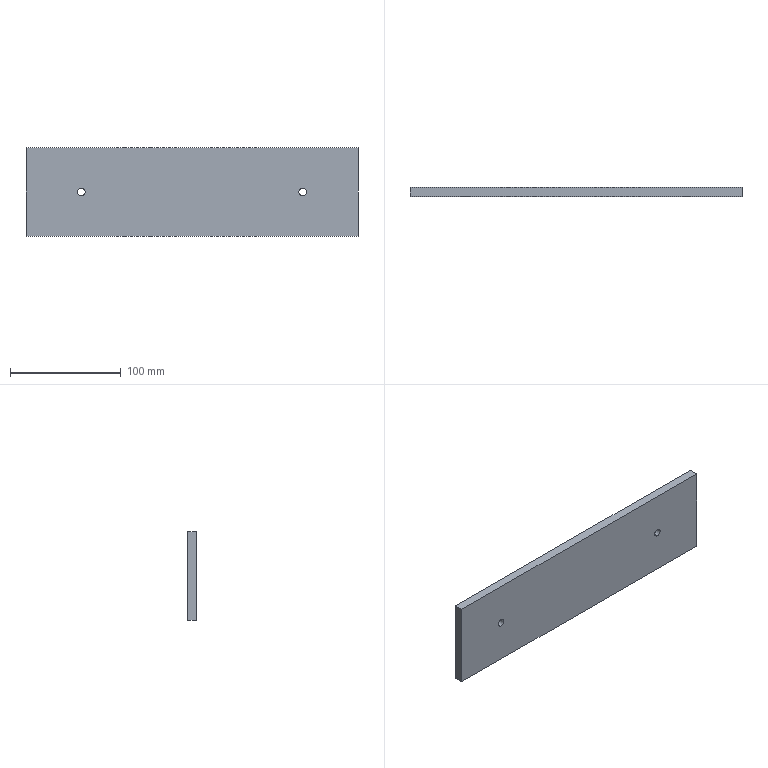Part | SolidWorks | features Extrusion 1, HoleWzd 1 | 1 solid | 10 faces | box 300 x 8 x 80 mm | volume 191419 mm3 | plane 6 | cylinder 4 | commonest cylinder face diameters 6.8 x4
STEP:
#1=CARTESIAN_POINT('',(50.,0.,-43.4));
#2=VERTEX_POINT('',#1);
#3=CARTESIAN_POINT('',(50.,0.,-36.6));
#4=VERTEX_POINT('',#3);
#5=CARTESIAN_POINT('',(50.,0.,-40.));
#6=DIRECTION('',(0.,1.,0.));
#7=DIRECTION('',(0.,0.,1.));
#8=AXIS2_PLACEMENT_3D('',#5,#6,#7);
#9=CIRCLE('',#8,3.4);
#10=EDGE_CURVE('',#2,#4,#9,.T.);
#11=ORIENTED_EDGE('',*,*,#10,.F.);
#12=CARTESIAN_POINT('',(50.,8.,-43.4));
#13=VERTEX_POINT('',#12);
#14=CARTESIAN_POINT('',(50.,8.,-43.4));
#15=DIRECTION('',(0.,1.,0.));
#16=VECTOR('',#15,1000.);
#17=LINE('',#14,#16);
#18=EDGE_CURVE('',#2,#13,#17,.T.);
#19=ORIENTED_EDGE('',*,*,#18,.T.);
#20=CARTESIAN_POINT('',(50.,8.,-36.6));
#21=VERTEX_POINT('',#20);
#22=CARTESIAN_POINT('',(50.,8.,-40.));
#23=DIRECTION('',(0.,1.,0.));
#24=DIRECTION('',(0.,0.,1.));
#25=AXIS2_PLACEMENT_3D('',#22,#23,#24);
#26=CIRCLE('',#25,3.4);
#27=EDGE_CURVE('',#13,#21,#26,.T.);
#28=ORIENTED_EDGE('',*,*,#27,.T.);
#29=CARTESIAN_POINT('',(50.,8.,-36.6));
#30=DIRECTION('',(0.,1.,0.));
#31=VECTOR('',#30,1000.);
#32=LINE('',#29,#31);
#33=EDGE_CURVE('',#4,#21,#32,.T.);
#34=ORIENTED_EDGE('',*,*,#33,.F.);
#35=EDGE_LOOP('',(#11,#19,#28,#34));
#36=FACE_OUTER_BOUND('',#35,.T.);
#37=CARTESIAN_POINT('',(50.,8.,-40.));
#38=DIRECTION('',(0.,1.,0.));
#39=DIRECTION('',(0.,0.,1.));
#40=AXIS2_PLACEMENT_3D('',#37,#38,#39);
#41=CYLINDRICAL_SURFACE('',#40,3.4);
#42=ADVANCED_FACE('',(#36),#41,.F.);
#43=CARTESIAN_POINT('',(250.,0.,-43.4));
#44=VERTEX_POINT('',#43);
#45=CARTESIAN_POINT('',(250.,0.,-36.6));
#46=VERTEX_POINT('',#45);
#47=CARTESIAN_POINT('',(250.,0.,-40.));
#48=DIRECTION('',(0.,1.,0.));
#49=DIRECTION('',(0.,0.,1.));
#50=AXIS2_PLACEMENT_3D('',#47,#48,#49);
#51=CIRCLE('',#50,3.4);
#52=EDGE_CURVE('',#44,#46,#51,.T.);
#53=ORIENTED_EDGE('',*,*,#52,.F.);
#54=CARTESIAN_POINT('',(250.,8.,-43.4));
#55=VERTEX_POINT('',#54);
#56=CARTESIAN_POINT('',(250.,8.,-43.4));
#57=DIRECTION('',(0.,1.,0.));
#58=VECTOR('',#57,1000.);
#59=LINE('',#56,#58);
#60=EDGE_CURVE('',#44,#55,#59,.T.);
#61=ORIENTED_EDGE('',*,*,#60,.T.);
#62=CARTESIAN_POINT('',(250.,8.,-36.6));
#63=VERTEX_POINT('',#62);
#64=CARTESIAN_POINT('',(250.,8.,-40.));
#65=DIRECTION('',(0.,1.,0.));
#66=DIRECTION('',(0.,0.,1.));
#67=AXIS2_PLACEMENT_3D('',#64,#65,#66);
#68=CIRCLE('',#67,3.4);
#69=EDGE_CURVE('',#55,#63,#68,.T.);
#70=ORIENTED_EDGE('',*,*,#69,.T.);
#71=CARTESIAN_POINT('',(250.,8.,-36.6));
#72=DIRECTION('',(0.,1.,0.));
#73=VECTOR('',#72,1000.);
#74=LINE('',#71,#73);
#75=EDGE_CURVE('',#46,#63,#74,.T.);
#76=ORIENTED_EDGE('',*,*,#75,.F.);
#77=EDGE_LOOP('',(#53,#61,#70,#76));
#78=FACE_OUTER_BOUND('',#77,.T.);
#79=CARTESIAN_POINT('',(250.,8.,-40.));
#80=DIRECTION('',(0.,1.,0.));
#81=DIRECTION('',(0.,0.,1.));
#82=AXIS2_PLACEMENT_3D('',#79,#80,#81);
#83=CYLINDRICAL_SURFACE('',#82,3.4);
#84=ADVANCED_FACE('',(#78),#83,.F.);
#85=CARTESIAN_POINT('',(0.,0.,-80.));
#86=VERTEX_POINT('',#85);
#87=CARTESIAN_POINT('',(0.,0.,0.));
#88=VERTEX_POINT('',#87);
#89=CARTESIAN_POINT('',(0.,0.,0.));
#90=DIRECTION('',(0.,0.,1.));
#91=VECTOR('',#90,1000.);
#92=LINE('',#89,#91);
#93=EDGE_CURVE('',#86,#88,#92,.T.);
#94=ORIENTED_EDGE('',*,*,#93,.T.);
#95=CARTESIAN_POINT('',(0.,8.,0.));
#96=VERTEX_POINT('',#95);
#97=CARTESIAN_POINT('',(0.,8.,0.));
#98=DIRECTION('',(0.,-1.,0.));
#99=VECTOR('',#98,1000.);
#100=LINE('',#97,#99);
#101=EDGE_CURVE('',#96,#88,#100,.T.);
#102=ORIENTED_EDGE('',*,*,#101,.F.);
#103=CARTESIAN_POINT('',(0.,8.,-80.));
#104=VERTEX_POINT('',#103);
#105=CARTESIAN_POINT('',(0.,8.,0.));
#106=DIRECTION('',(0.,0.,1.));
#107=VECTOR('',#106,1000.);
#108=LINE('',#105,#107);
#109=EDGE_CURVE('',#104,#96,#108,.T.);
#110=ORIENTED_EDGE('',*,*,#109,.F.);
#111=CARTESIAN_POINT('',(0.,8.,-80.));
#112=DIRECTION('',(0.,-1.,0.));
#113=VECTOR('',#112,1000.);
#114=LINE('',#111,#113);
#115=EDGE_CURVE('',#104,#86,#114,.T.);
#116=ORIENTED_EDGE('',*,*,#115,.T.);
#117=EDGE_LOOP('',(#94,#102,#110,#116));
#118=FACE_OUTER_BOUND('',#117,.T.);
#119=CARTESIAN_POINT('',(0.,8.,0.));
#120=DIRECTION('',(1.,0.,0.));
#121=DIRECTION('',(0.,0.,-1.));
#122=AXIS2_PLACEMENT_3D('',#119,#120,#121);
#123=PLANE('',#122);
#124=ADVANCED_FACE('',(#118),#123,.F.);
#125=CARTESIAN_POINT('',(300.,0.,0.));
#126=VERTEX_POINT('',#125);
#127=CARTESIAN_POINT('',(0.,0.,0.));
#128=DIRECTION('',(1.,0.,0.));
#129=VECTOR('',#128,1000.);
#130=LINE('',#127,#129);
#131=EDGE_CURVE('',#88,#126,#130,.T.);
#132=ORIENTED_EDGE('',*,*,#131,.T.);
#133=CARTESIAN_POINT('',(300.,8.,0.));
#134=VERTEX_POINT('',#133);
#135=CARTESIAN_POINT('',(300.,8.,0.));
#136=DIRECTION('',(0.,-1.,0.));
#137=VECTOR('',#136,1000.);
#138=LINE('',#135,#137);
#139=EDGE_CURVE('',#134,#126,#138,.T.);
#140=ORIENTED_EDGE('',*,*,#139,.F.);
#141=CARTESIAN_POINT('',(0.,8.,0.));
#142=DIRECTION('',(1.,0.,0.));
#143=VECTOR('',#142,1000.);
#144=LINE('',#141,#143);
#145=EDGE_CURVE('',#96,#134,#144,.T.);
#146=ORIENTED_EDGE('',*,*,#145,.F.);
#147=ORIENTED_EDGE('',*,*,#101,.T.);
#148=EDGE_LOOP('',(#132,#140,#146,#147));
#149=FACE_OUTER_BOUND('',#148,.T.);
#150=CARTESIAN_POINT('',(0.,8.,0.));
#151=DIRECTION('',(0.,0.,-1.));
#152=DIRECTION('',(-1.,0.,0.));
#153=AXIS2_PLACEMENT_3D('',#150,#151,#152);
#154=PLANE('',#153);
#155=ADVANCED_FACE('',(#149),#154,.F.);
#156=CARTESIAN_POINT('',(300.,0.,-80.));
#157=VERTEX_POINT('',#156);
#158=CARTESIAN_POINT('',(300.,0.,0.));
#159=DIRECTION('',(0.,0.,-1.));
#160=VECTOR('',#159,1000.);
#161=LINE('',#158,#160);
#162=EDGE_CURVE('',#126,#157,#161,.T.);
#163=ORIENTED_EDGE('',*,*,#162,.T.);
#164=CARTESIAN_POINT('',(300.,8.,-80.));
#165=VERTEX_POINT('',#164);
#166=CARTESIAN_POINT('',(300.,8.,-80.));
#167=DIRECTION('',(0.,-1.,0.));
#168=VECTOR('',#167,1000.);
#169=LINE('',#166,#168);
#170=EDGE_CURVE('',#165,#157,#169,.T.);
#171=ORIENTED_EDGE('',*,*,#170,.F.);
#172=CARTESIAN_POINT('',(300.,8.,0.));
#173=DIRECTION('',(0.,0.,-1.));
#174=VECTOR('',#173,1000.);
#175=LINE('',#172,#174);
#176=EDGE_CURVE('',#134,#165,#175,.T.);
#177=ORIENTED_EDGE('',*,*,#176,.F.);
#178=ORIENTED_EDGE('',*,*,#139,.T.);
#179=EDGE_LOOP('',(#163,#171,#177,#178));
#180=FACE_OUTER_BOUND('',#179,.T.);
#181=CARTESIAN_POINT('',(300.,8.,0.));
#182=DIRECTION('',(-1.,0.,0.));
#183=DIRECTION('',(0.,0.,1.));
#184=AXIS2_PLACEMENT_3D('',#181,#182,#183);
#185=PLANE('',#184);
#186=ADVANCED_FACE('',(#180),#185,.F.);
#187=CARTESIAN_POINT('',(0.,0.,-80.));
#188=DIRECTION('',(-1.,0.,0.));
#189=VECTOR('',#188,1000.);
#190=LINE('',#187,#189);
#191=EDGE_CURVE('',#157,#86,#190,.T.);
#192=ORIENTED_EDGE('',*,*,#191,.T.);
#193=ORIENTED_EDGE('',*,*,#115,.F.);
#194=CARTESIAN_POINT('',(0.,8.,-80.));
#195=DIRECTION('',(-1.,0.,0.));
#196=VECTOR('',#195,1000.);
#197=LINE('',#194,#196);
#198=EDGE_CURVE('',#165,#104,#197,.T.);
#199=ORIENTED_EDGE('',*,*,#198,.F.);
#200=ORIENTED_EDGE('',*,*,#170,.T.);
#201=EDGE_LOOP('',(#192,#193,#199,#200));
#202=FACE_OUTER_BOUND('',#201,.T.);
#203=CARTESIAN_POINT('',(0.,8.,-80.));
#204=DIRECTION('',(0.,0.,1.));
#205=DIRECTION('',(1.,0.,0.));
#206=AXIS2_PLACEMENT_3D('',#203,#204,#205);
#207=PLANE('',#206);
#208=ADVANCED_FACE('',(#202),#207,.F.);
#209=CARTESIAN_POINT('',(50.,8.,-40.));
#210=DIRECTION('',(0.,1.,0.));
#211=DIRECTION('',(0.,0.,1.));
#212=AXIS2_PLACEMENT_3D('',#209,#210,#211);
#213=CIRCLE('',#212,3.4);
#214=EDGE_CURVE('',#21,#13,#213,.T.);
#215=ORIENTED_EDGE('',*,*,#214,.F.);
#216=ORIENTED_EDGE('',*,*,#27,.F.);
#217=EDGE_LOOP('',(#215,#216));
#218=FACE_BOUND('',#217,.T.);
#219=CARTESIAN_POINT('',(250.,8.,-40.));
#220=DIRECTION('',(0.,1.,0.));
#221=DIRECTION('',(0.,0.,1.));
#222=AXIS2_PLACEMENT_3D('',#219,#220,#221);
#223=CIRCLE('',#222,3.4);
#224=EDGE_CURVE('',#63,#55,#223,.T.);
#225=ORIENTED_EDGE('',*,*,#224,.F.);
#226=ORIENTED_EDGE('',*,*,#69,.F.);
#227=EDGE_LOOP('',(#225,#226));
#228=FACE_BOUND('',#227,.T.);
#229=ORIENTED_EDGE('',*,*,#109,.T.);
#230=ORIENTED_EDGE('',*,*,#145,.T.);
#231=ORIENTED_EDGE('',*,*,#176,.T.);
#232=ORIENTED_EDGE('',*,*,#198,.T.);
#233=EDGE_LOOP('',(#229,#230,#231,#232));
#234=FACE_OUTER_BOUND('',#233,.T.);
#235=CARTESIAN_POINT('',(0.,8.,0.));
#236=DIRECTION('',(0.,-1.,0.));
#237=DIRECTION('',(0.,0.,-1.));
#238=AXIS2_PLACEMENT_3D('',#235,#236,#237);
#239=PLANE('',#238);
#240=ADVANCED_FACE('',(#218,#228,#234),#239,.F.);
#241=CARTESIAN_POINT('',(50.,0.,-40.));
#242=DIRECTION('',(0.,1.,0.));
#243=DIRECTION('',(0.,0.,1.));
#244=AXIS2_PLACEMENT_3D('',#241,#242,#243);
#245=CIRCLE('',#244,3.4);
#246=EDGE_CURVE('',#4,#2,#245,.T.);
#247=ORIENTED_EDGE('',*,*,#246,.T.);
#248=ORIENTED_EDGE('',*,*,#10,.T.);
#249=EDGE_LOOP('',(#247,#248));
#250=FACE_BOUND('',#249,.T.);
#251=CARTESIAN_POINT('',(250.,0.,-40.));
#252=DIRECTION('',(0.,1.,0.));
#253=DIRECTION('',(0.,0.,1.));
#254=AXIS2_PLACEMENT_3D('',#251,#252,#253);
#255=CIRCLE('',#254,3.4);
#256=EDGE_CURVE('',#46,#44,#255,.T.);
#257=ORIENTED_EDGE('',*,*,#256,.T.);
#258=ORIENTED_EDGE('',*,*,#52,.T.);
#259=EDGE_LOOP('',(#257,#258));
#260=FACE_BOUND('',#259,.T.);
#261=ORIENTED_EDGE('',*,*,#93,.F.);
#262=ORIENTED_EDGE('',*,*,#191,.F.);
#263=ORIENTED_EDGE('',*,*,#162,.F.);
#264=ORIENTED_EDGE('',*,*,#131,.F.);
#265=EDGE_LOOP('',(#261,#262,#263,#264));
#266=FACE_OUTER_BOUND('',#265,.T.);
#267=CARTESIAN_POINT('',(0.,0.,0.));
#268=DIRECTION('',(0.,-1.,0.));
#269=DIRECTION('',(0.,0.,-1.));
#270=AXIS2_PLACEMENT_3D('',#267,#268,#269);
#271=PLANE('',#270);
#272=ADVANCED_FACE('',(#250,#260,#266),#271,.T.);
#273=ORIENTED_EDGE('',*,*,#60,.F.);
#274=ORIENTED_EDGE('',*,*,#256,.F.);
#275=ORIENTED_EDGE('',*,*,#75,.T.);
#276=ORIENTED_EDGE('',*,*,#224,.T.);
#277=EDGE_LOOP('',(#273,#274,#275,#276));
#278=FACE_OUTER_BOUND('',#277,.T.);
#279=CARTESIAN_POINT('',(250.,8.,-40.));
#280=DIRECTION('',(0.,1.,0.));
#281=DIRECTION('',(0.,0.,1.));
#282=AXIS2_PLACEMENT_3D('',#279,#280,#281);
#283=CYLINDRICAL_SURFACE('',#282,3.4);
#284=ADVANCED_FACE('',(#278),#283,.F.);
#285=ORIENTED_EDGE('',*,*,#18,.F.);
#286=ORIENTED_EDGE('',*,*,#246,.F.);
#287=ORIENTED_EDGE('',*,*,#33,.T.);
#288=ORIENTED_EDGE('',*,*,#214,.T.);
#289=EDGE_LOOP('',(#285,#286,#287,#288));
#290=FACE_OUTER_BOUND('',#289,.T.);
#291=CARTESIAN_POINT('',(50.,8.,-40.));
#292=DIRECTION('',(0.,1.,0.));
#293=DIRECTION('',(0.,0.,1.));
#294=AXIS2_PLACEMENT_3D('',#291,#292,#293);
#295=CYLINDRICAL_SURFACE('',#294,3.4);
#296=ADVANCED_FACE('',(#290),#295,.F.);
#297=CLOSED_SHELL('',(#42,#84,#124,#155,#186,#208,#240,#272,#284,#296));
#298=MANIFOLD_SOLID_BREP('',#297);
#299=CARTESIAN_POINT('',(0.,0.,0.));
#300=DIRECTION('',(0.,0.,1.));
#301=DIRECTION('',(1.,0.,0.));
#302=AXIS2_PLACEMENT_3D('',#299,#300,#301);
#303=(LENGTH_UNIT()NAMED_UNIT(*)SI_UNIT(.MILLI.,.METRE.));
#304=UNCERTAINTY_MEASURE_WITH_UNIT(LENGTH_MEASURE(0.00001),#303,'','');
#305=(NAMED_UNIT(*)PLANE_ANGLE_UNIT()SI_UNIT($,.RADIAN.));
#306=(NAMED_UNIT(*)SI_UNIT($,.STERADIAN.)SOLID_ANGLE_UNIT());
#307=(GEOMETRIC_REPRESENTATION_CONTEXT(3)GLOBAL_UNCERTAINTY_ASSIGNED_CONTEXT((#304))GLOBAL_UNIT_ASSIGNED_CONTEXT((#303,#305,#306))REPRESENTATION_CONTEXT('',''));
#308=ADVANCED_BREP_SHAPE_REPRESENTATION('',(#298,#302),#307);